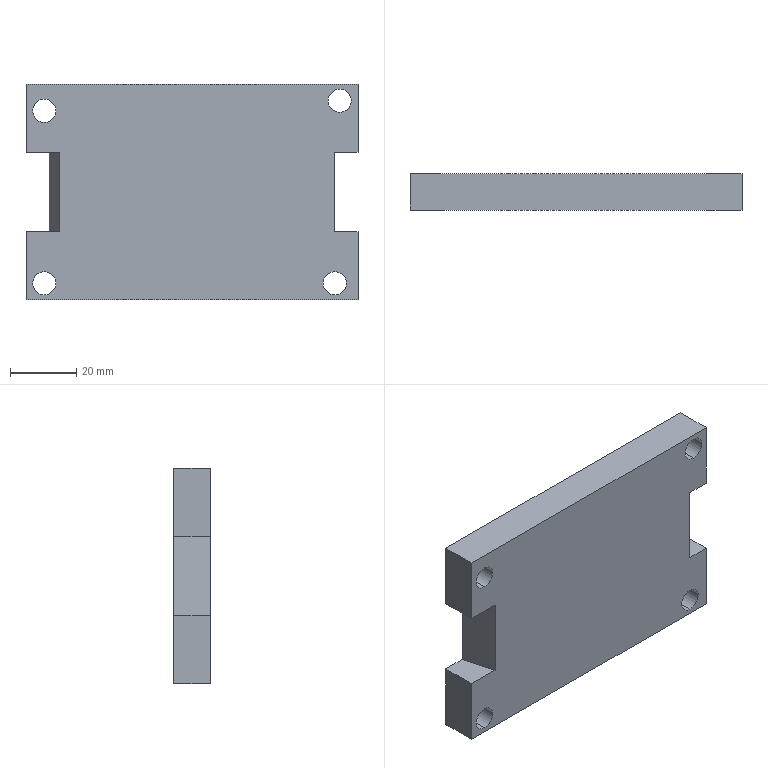Part | STEP file | X77ZZ-01001 | 1 solid | 22 faces | box 100 x 11 x 65 mm | volume 65319 mm3 | plane 14 | cylinder 8 | commonest cylinder face diameters 7 x8
STEP:
#1=CARTESIAN_POINT('',(-44.5,0.,-31.));
#2=VERTEX_POINT('',#1);
#3=CARTESIAN_POINT('',(-44.5,0.,-24.));
#4=VERTEX_POINT('',#3);
#5=CARTESIAN_POINT('',(-44.5,0.,-27.5));
#6=DIRECTION('',(0.,1.,0.));
#7=DIRECTION('',(0.,0.,1.));
#8=AXIS2_PLACEMENT_3D('',#5,#6,#7);
#9=CIRCLE('',#8,3.5);
#10=EDGE_CURVE('',#2,#4,#9,.T.);
#11=ORIENTED_EDGE('',*,*,#10,.F.);
#12=CARTESIAN_POINT('',(-44.5,11.,-31.));
#13=VERTEX_POINT('',#12);
#14=CARTESIAN_POINT('',(-44.5,0.,-31.));
#15=DIRECTION('',(0.,1.,0.));
#16=VECTOR('',#15,1000.);
#17=LINE('',#14,#16);
#18=EDGE_CURVE('',#2,#13,#17,.T.);
#19=ORIENTED_EDGE('',*,*,#18,.T.);
#20=CARTESIAN_POINT('',(-44.5,11.,-24.));
#21=VERTEX_POINT('',#20);
#22=CARTESIAN_POINT('',(-44.5,11.,-27.5));
#23=DIRECTION('',(0.,1.,0.));
#24=DIRECTION('',(0.,0.,1.));
#25=AXIS2_PLACEMENT_3D('',#22,#23,#24);
#26=CIRCLE('',#25,3.5);
#27=EDGE_CURVE('',#13,#21,#26,.T.);
#28=ORIENTED_EDGE('',*,*,#27,.T.);
#29=CARTESIAN_POINT('',(-44.5,0.,-24.));
#30=DIRECTION('',(0.,1.,0.));
#31=VECTOR('',#30,1000.);
#32=LINE('',#29,#31);
#33=EDGE_CURVE('',#4,#21,#32,.T.);
#34=ORIENTED_EDGE('',*,*,#33,.F.);
#35=EDGE_LOOP('',(#11,#19,#28,#34));
#36=FACE_OUTER_BOUND('',#35,.T.);
#37=CARTESIAN_POINT('',(-44.5,0.,-27.5));
#38=DIRECTION('',(0.,1.,0.));
#39=DIRECTION('',(0.,0.,1.));
#40=AXIS2_PLACEMENT_3D('',#37,#38,#39);
#41=CYLINDRICAL_SURFACE('',#40,3.5);
#42=ADVANCED_FACE('',(#36),#41,.F.);
#43=CARTESIAN_POINT('',(43.014,0.,-31.));
#44=VERTEX_POINT('',#43);
#45=CARTESIAN_POINT('',(43.014,0.,-24.));
#46=VERTEX_POINT('',#45);
#47=CARTESIAN_POINT('',(43.014,0.,-27.5));
#48=DIRECTION('',(0.,1.,0.));
#49=DIRECTION('',(0.,0.,1.));
#50=AXIS2_PLACEMENT_3D('',#47,#48,#49);
#51=CIRCLE('',#50,3.5);
#52=EDGE_CURVE('',#44,#46,#51,.T.);
#53=ORIENTED_EDGE('',*,*,#52,.F.);
#54=CARTESIAN_POINT('',(43.014,11.,-31.));
#55=VERTEX_POINT('',#54);
#56=CARTESIAN_POINT('',(43.014,0.,-31.));
#57=DIRECTION('',(0.,1.,0.));
#58=VECTOR('',#57,1000.);
#59=LINE('',#56,#58);
#60=EDGE_CURVE('',#44,#55,#59,.T.);
#61=ORIENTED_EDGE('',*,*,#60,.T.);
#62=CARTESIAN_POINT('',(43.014,11.,-24.));
#63=VERTEX_POINT('',#62);
#64=CARTESIAN_POINT('',(43.014,11.,-27.5));
#65=DIRECTION('',(0.,1.,0.));
#66=DIRECTION('',(0.,0.,1.));
#67=AXIS2_PLACEMENT_3D('',#64,#65,#66);
#68=CIRCLE('',#67,3.5);
#69=EDGE_CURVE('',#55,#63,#68,.T.);
#70=ORIENTED_EDGE('',*,*,#69,.T.);
#71=CARTESIAN_POINT('',(43.014,0.,-24.));
#72=DIRECTION('',(0.,1.,0.));
#73=VECTOR('',#72,1000.);
#74=LINE('',#71,#73);
#75=EDGE_CURVE('',#46,#63,#74,.T.);
#76=ORIENTED_EDGE('',*,*,#75,.F.);
#77=EDGE_LOOP('',(#53,#61,#70,#76));
#78=FACE_OUTER_BOUND('',#77,.T.);
#79=CARTESIAN_POINT('',(43.014,0.,-27.5));
#80=DIRECTION('',(0.,1.,0.));
#81=DIRECTION('',(0.,0.,1.));
#82=AXIS2_PLACEMENT_3D('',#79,#80,#81);
#83=CYLINDRICAL_SURFACE('',#82,3.5);
#84=ADVANCED_FACE('',(#78),#83,.F.);
#85=CARTESIAN_POINT('',(-44.5,0.,20.979));
#86=VERTEX_POINT('',#85);
#87=CARTESIAN_POINT('',(-44.5,0.,27.979));
#88=VERTEX_POINT('',#87);
#89=CARTESIAN_POINT('',(-44.5,0.,24.479));
#90=DIRECTION('',(0.,1.,0.));
#91=DIRECTION('',(0.,0.,1.));
#92=AXIS2_PLACEMENT_3D('',#89,#90,#91);
#93=CIRCLE('',#92,3.5);
#94=EDGE_CURVE('',#86,#88,#93,.T.);
#95=ORIENTED_EDGE('',*,*,#94,.F.);
#96=CARTESIAN_POINT('',(-44.5,11.,20.979));
#97=VERTEX_POINT('',#96);
#98=CARTESIAN_POINT('',(-44.5,0.,20.979));
#99=DIRECTION('',(0.,1.,0.));
#100=VECTOR('',#99,1000.);
#101=LINE('',#98,#100);
#102=EDGE_CURVE('',#86,#97,#101,.T.);
#103=ORIENTED_EDGE('',*,*,#102,.T.);
#104=CARTESIAN_POINT('',(-44.5,11.,27.979));
#105=VERTEX_POINT('',#104);
#106=CARTESIAN_POINT('',(-44.5,11.,24.479));
#107=DIRECTION('',(0.,1.,0.));
#108=DIRECTION('',(0.,0.,1.));
#109=AXIS2_PLACEMENT_3D('',#106,#107,#108);
#110=CIRCLE('',#109,3.5);
#111=EDGE_CURVE('',#97,#105,#110,.T.);
#112=ORIENTED_EDGE('',*,*,#111,.T.);
#113=CARTESIAN_POINT('',(-44.5,0.,27.979));
#114=DIRECTION('',(0.,1.,0.));
#115=VECTOR('',#114,1000.);
#116=LINE('',#113,#115);
#117=EDGE_CURVE('',#88,#105,#116,.T.);
#118=ORIENTED_EDGE('',*,*,#117,.F.);
#119=EDGE_LOOP('',(#95,#103,#112,#118));
#120=FACE_OUTER_BOUND('',#119,.T.);
#121=CARTESIAN_POINT('',(-44.5,0.,24.479));
#122=DIRECTION('',(0.,1.,0.));
#123=DIRECTION('',(0.,0.,1.));
#124=AXIS2_PLACEMENT_3D('',#121,#122,#123);
#125=CYLINDRICAL_SURFACE('',#124,3.5);
#126=ADVANCED_FACE('',(#120),#125,.F.);
#127=CARTESIAN_POINT('',(44.5,0.,24.));
#128=VERTEX_POINT('',#127);
#129=CARTESIAN_POINT('',(44.5,0.,31.));
#130=VERTEX_POINT('',#129);
#131=CARTESIAN_POINT('',(44.5,0.,27.5));
#132=DIRECTION('',(0.,1.,0.));
#133=DIRECTION('',(0.,0.,1.));
#134=AXIS2_PLACEMENT_3D('',#131,#132,#133);
#135=CIRCLE('',#134,3.5);
#136=EDGE_CURVE('',#128,#130,#135,.T.);
#137=ORIENTED_EDGE('',*,*,#136,.F.);
#138=CARTESIAN_POINT('',(44.5,11.,24.));
#139=VERTEX_POINT('',#138);
#140=CARTESIAN_POINT('',(44.5,0.,24.));
#141=DIRECTION('',(0.,1.,0.));
#142=VECTOR('',#141,1000.);
#143=LINE('',#140,#142);
#144=EDGE_CURVE('',#128,#139,#143,.T.);
#145=ORIENTED_EDGE('',*,*,#144,.T.);
#146=CARTESIAN_POINT('',(44.5,11.,31.));
#147=VERTEX_POINT('',#146);
#148=CARTESIAN_POINT('',(44.5,11.,27.5));
#149=DIRECTION('',(0.,1.,0.));
#150=DIRECTION('',(0.,0.,1.));
#151=AXIS2_PLACEMENT_3D('',#148,#149,#150);
#152=CIRCLE('',#151,3.5);
#153=EDGE_CURVE('',#139,#147,#152,.T.);
#154=ORIENTED_EDGE('',*,*,#153,.T.);
#155=CARTESIAN_POINT('',(44.5,0.,31.));
#156=DIRECTION('',(0.,1.,0.));
#157=VECTOR('',#156,1000.);
#158=LINE('',#155,#157);
#159=EDGE_CURVE('',#130,#147,#158,.T.);
#160=ORIENTED_EDGE('',*,*,#159,.F.);
#161=EDGE_LOOP('',(#137,#145,#154,#160));
#162=FACE_OUTER_BOUND('',#161,.T.);
#163=CARTESIAN_POINT('',(44.5,0.,27.5));
#164=DIRECTION('',(0.,1.,0.));
#165=DIRECTION('',(0.,0.,1.));
#166=AXIS2_PLACEMENT_3D('',#163,#164,#165);
#167=CYLINDRICAL_SURFACE('',#166,3.5);
#168=ADVANCED_FACE('',(#162),#167,.F.);
#169=CARTESIAN_POINT('',(-44.5,11.,-27.5));
#170=DIRECTION('',(0.,1.,0.));
#171=DIRECTION('',(0.,0.,1.));
#172=AXIS2_PLACEMENT_3D('',#169,#170,#171);
#173=CIRCLE('',#172,3.5);
#174=EDGE_CURVE('',#21,#13,#173,.T.);
#175=ORIENTED_EDGE('',*,*,#174,.F.);
#176=ORIENTED_EDGE('',*,*,#27,.F.);
#177=EDGE_LOOP('',(#175,#176));
#178=FACE_BOUND('',#177,.T.);
#179=CARTESIAN_POINT('',(43.014,11.,-27.5));
#180=DIRECTION('',(0.,1.,0.));
#181=DIRECTION('',(0.,0.,1.));
#182=AXIS2_PLACEMENT_3D('',#179,#180,#181);
#183=CIRCLE('',#182,3.5);
#184=EDGE_CURVE('',#63,#55,#183,.T.);
#185=ORIENTED_EDGE('',*,*,#184,.F.);
#186=ORIENTED_EDGE('',*,*,#69,.F.);
#187=EDGE_LOOP('',(#185,#186));
#188=FACE_BOUND('',#187,.T.);
#189=CARTESIAN_POINT('',(-44.5,11.,24.479));
#190=DIRECTION('',(0.,1.,0.));
#191=DIRECTION('',(0.,0.,1.));
#192=AXIS2_PLACEMENT_3D('',#189,#190,#191);
#193=CIRCLE('',#192,3.5);
#194=EDGE_CURVE('',#105,#97,#193,.T.);
#195=ORIENTED_EDGE('',*,*,#194,.F.);
#196=ORIENTED_EDGE('',*,*,#111,.F.);
#197=EDGE_LOOP('',(#195,#196));
#198=FACE_BOUND('',#197,.T.);
#199=CARTESIAN_POINT('',(44.5,11.,27.5));
#200=DIRECTION('',(0.,1.,0.));
#201=DIRECTION('',(0.,0.,1.));
#202=AXIS2_PLACEMENT_3D('',#199,#200,#201);
#203=CIRCLE('',#202,3.5);
#204=EDGE_CURVE('',#147,#139,#203,.T.);
#205=ORIENTED_EDGE('',*,*,#204,.F.);
#206=ORIENTED_EDGE('',*,*,#153,.F.);
#207=EDGE_LOOP('',(#205,#206));
#208=FACE_BOUND('',#207,.T.);
#209=CARTESIAN_POINT('',(-43.,11.,12.));
#210=VERTEX_POINT('',#209);
#211=CARTESIAN_POINT('',(-50.,11.,12.));
#212=VERTEX_POINT('',#211);
#213=CARTESIAN_POINT('',(-50.,11.,12.));
#214=DIRECTION('',(-1.,0.,0.));
#215=VECTOR('',#214,1000.);
#216=LINE('',#213,#215);
#217=EDGE_CURVE('',#210,#212,#216,.T.);
#218=ORIENTED_EDGE('',*,*,#217,.T.);
#219=CARTESIAN_POINT('',(-50.,11.,32.5));
#220=VERTEX_POINT('',#219);
#221=CARTESIAN_POINT('',(-50.,11.,32.5));
#222=DIRECTION('',(0.,0.,1.));
#223=VECTOR('',#222,1000.);
#224=LINE('',#221,#223);
#225=EDGE_CURVE('',#212,#220,#224,.T.);
#226=ORIENTED_EDGE('',*,*,#225,.T.);
#227=CARTESIAN_POINT('',(50.,11.,32.5));
#228=VERTEX_POINT('',#227);
#229=CARTESIAN_POINT('',(-50.,11.,32.5));
#230=DIRECTION('',(1.,0.,0.));
#231=VECTOR('',#230,1000.);
#232=LINE('',#229,#231);
#233=EDGE_CURVE('',#220,#228,#232,.T.);
#234=ORIENTED_EDGE('',*,*,#233,.T.);
#235=CARTESIAN_POINT('',(50.,11.,12.));
#236=VERTEX_POINT('',#235);
#237=CARTESIAN_POINT('',(50.,11.,32.5));
#238=DIRECTION('',(0.,0.,-1.));
#239=VECTOR('',#238,1000.);
#240=LINE('',#237,#239);
#241=EDGE_CURVE('',#228,#236,#240,.T.);
#242=ORIENTED_EDGE('',*,*,#241,.T.);
#243=CARTESIAN_POINT('',(40.,11.,12.));
#244=VERTEX_POINT('',#243);
#245=CARTESIAN_POINT('',(40.,11.,12.));
#246=DIRECTION('',(-1.,0.,0.));
#247=VECTOR('',#246,1000.);
#248=LINE('',#245,#247);
#249=EDGE_CURVE('',#236,#244,#248,.T.);
#250=ORIENTED_EDGE('',*,*,#249,.T.);
#251=CARTESIAN_POINT('',(40.,11.,-12.));
#252=VERTEX_POINT('',#251);
#253=CARTESIAN_POINT('',(40.,11.,12.));
#254=DIRECTION('',(0.,0.,-1.));
#255=VECTOR('',#254,1000.);
#256=LINE('',#253,#255);
#257=EDGE_CURVE('',#244,#252,#256,.T.);
#258=ORIENTED_EDGE('',*,*,#257,.T.);
#259=CARTESIAN_POINT('',(50.,11.,-12.));
#260=VERTEX_POINT('',#259);
#261=CARTESIAN_POINT('',(40.,11.,-12.));
#262=DIRECTION('',(-1.,0.,0.));
#263=VECTOR('',#262,1000.);
#264=LINE('',#261,#263);
#265=EDGE_CURVE('',#260,#252,#264,.T.);
#266=ORIENTED_EDGE('',*,*,#265,.F.);
#267=CARTESIAN_POINT('',(50.,11.,-32.5));
#268=VERTEX_POINT('',#267);
#269=CARTESIAN_POINT('',(50.,11.,32.5));
#270=DIRECTION('',(0.,0.,-1.));
#271=VECTOR('',#270,1000.);
#272=LINE('',#269,#271);
#273=EDGE_CURVE('',#260,#268,#272,.T.);
#274=ORIENTED_EDGE('',*,*,#273,.T.);
#275=CARTESIAN_POINT('',(-50.,11.,-32.5));
#276=VERTEX_POINT('',#275);
#277=CARTESIAN_POINT('',(-50.,11.,-32.5));
#278=DIRECTION('',(-1.,0.,0.));
#279=VECTOR('',#278,1000.);
#280=LINE('',#277,#279);
#281=EDGE_CURVE('',#268,#276,#280,.T.);
#282=ORIENTED_EDGE('',*,*,#281,.T.);
#283=CARTESIAN_POINT('',(-50.,11.,-12.));
#284=VERTEX_POINT('',#283);
#285=CARTESIAN_POINT('',(-50.,11.,32.5));
#286=DIRECTION('',(0.,0.,1.));
#287=VECTOR('',#286,1000.);
#288=LINE('',#285,#287);
#289=EDGE_CURVE('',#276,#284,#288,.T.);
#290=ORIENTED_EDGE('',*,*,#289,.T.);
#291=CARTESIAN_POINT('',(-43.,11.,-12.));
#292=VERTEX_POINT('',#291);
#293=CARTESIAN_POINT('',(-50.,11.,-12.));
#294=DIRECTION('',(-1.,0.,0.));
#295=VECTOR('',#294,1000.);
#296=LINE('',#293,#295);
#297=EDGE_CURVE('',#292,#284,#296,.T.);
#298=ORIENTED_EDGE('',*,*,#297,.F.);
#299=CARTESIAN_POINT('',(-43.,11.,12.));
#300=DIRECTION('',(0.,0.,-1.));
#301=VECTOR('',#300,1000.);
#302=LINE('',#299,#301);
#303=EDGE_CURVE('',#210,#292,#302,.T.);
#304=ORIENTED_EDGE('',*,*,#303,.F.);
#305=EDGE_LOOP('',(#218,#226,#234,#242,#250,#258,#266,#274,#282,#290,#298,#304));
#306=FACE_OUTER_BOUND('',#305,.T.);
#307=CARTESIAN_POINT('',(50.,11.,-32.5));
#308=DIRECTION('',(0.,-1.,0.));
#309=DIRECTION('',(0.,0.,-1.));
#310=AXIS2_PLACEMENT_3D('',#307,#308,#309);
#311=PLANE('',#310);
#312=ADVANCED_FACE('',(#178,#188,#198,#208,#306),#311,.F.);
#313=CARTESIAN_POINT('',(-44.5,0.,-27.5));
#314=DIRECTION('',(0.,1.,0.));
#315=DIRECTION('',(0.,0.,1.));
#316=AXIS2_PLACEMENT_3D('',#313,#314,#315);
#317=CIRCLE('',#316,3.5);
#318=EDGE_CURVE('',#4,#2,#317,.T.);
#319=ORIENTED_EDGE('',*,*,#318,.T.);
#320=ORIENTED_EDGE('',*,*,#10,.T.);
#321=EDGE_LOOP('',(#319,#320));
#322=FACE_BOUND('',#321,.T.);
#323=CARTESIAN_POINT('',(43.014,0.,-27.5));
#324=DIRECTION('',(0.,1.,0.));
#325=DIRECTION('',(0.,0.,1.));
#326=AXIS2_PLACEMENT_3D('',#323,#324,#325);
#327=CIRCLE('',#326,3.5);
#328=EDGE_CURVE('',#46,#44,#327,.T.);
#329=ORIENTED_EDGE('',*,*,#328,.T.);
#330=ORIENTED_EDGE('',*,*,#52,.T.);
#331=EDGE_LOOP('',(#329,#330));
#332=FACE_BOUND('',#331,.T.);
#333=CARTESIAN_POINT('',(-44.5,0.,24.479));
#334=DIRECTION('',(0.,1.,0.));
#335=DIRECTION('',(0.,0.,1.));
#336=AXIS2_PLACEMENT_3D('',#333,#334,#335);
#337=CIRCLE('',#336,3.5);
#338=EDGE_CURVE('',#88,#86,#337,.T.);
#339=ORIENTED_EDGE('',*,*,#338,.T.);
#340=ORIENTED_EDGE('',*,*,#94,.T.);
#341=EDGE_LOOP('',(#339,#340));
#342=FACE_BOUND('',#341,.T.);
#343=CARTESIAN_POINT('',(44.5,0.,27.5));
#344=DIRECTION('',(0.,1.,0.));
#345=DIRECTION('',(0.,0.,1.));
#346=AXIS2_PLACEMENT_3D('',#343,#344,#345);
#347=CIRCLE('',#346,3.5);
#348=EDGE_CURVE('',#130,#128,#347,.T.);
#349=ORIENTED_EDGE('',*,*,#348,.T.);
#350=ORIENTED_EDGE('',*,*,#136,.T.);
#351=EDGE_LOOP('',(#349,#350));
#352=FACE_BOUND('',#351,.T.);
#353=CARTESIAN_POINT('',(-50.,0.,12.));
#354=VERTEX_POINT('',#353);
#355=CARTESIAN_POINT('',(-50.,0.,32.5));
#356=VERTEX_POINT('',#355);
#357=CARTESIAN_POINT('',(-50.,0.,32.5));
#358=DIRECTION('',(0.,0.,1.));
#359=VECTOR('',#358,1000.);
#360=LINE('',#357,#359);
#361=EDGE_CURVE('',#354,#356,#360,.T.);
#362=ORIENTED_EDGE('',*,*,#361,.F.);
#363=CARTESIAN_POINT('',(-40.,0.,12.));
#364=VERTEX_POINT('',#363);
#365=CARTESIAN_POINT('',(-40.,0.,12.));
#366=DIRECTION('',(1.,0.,0.));
#367=VECTOR('',#366,1000.);
#368=LINE('',#365,#367);
#369=EDGE_CURVE('',#354,#364,#368,.T.);
#370=ORIENTED_EDGE('',*,*,#369,.T.);
#371=CARTESIAN_POINT('',(-40.,0.,-12.));
#372=VERTEX_POINT('',#371);
#373=CARTESIAN_POINT('',(-40.,0.,12.));
#374=DIRECTION('',(0.,0.,-1.));
#375=VECTOR('',#374,1000.);
#376=LINE('',#373,#375);
#377=EDGE_CURVE('',#364,#372,#376,.T.);
#378=ORIENTED_EDGE('',*,*,#377,.T.);
#379=CARTESIAN_POINT('',(-50.,0.,-12.));
#380=VERTEX_POINT('',#379);
#381=CARTESIAN_POINT('',(-40.,0.,-12.));
#382=DIRECTION('',(1.,0.,0.));
#383=VECTOR('',#382,1000.);
#384=LINE('',#381,#383);
#385=EDGE_CURVE('',#380,#372,#384,.T.);
#386=ORIENTED_EDGE('',*,*,#385,.F.);
#387=CARTESIAN_POINT('',(-50.,0.,-32.5));
#388=VERTEX_POINT('',#387);
#389=CARTESIAN_POINT('',(-50.,0.,32.5));
#390=DIRECTION('',(0.,0.,1.));
#391=VECTOR('',#390,1000.);
#392=LINE('',#389,#391);
#393=EDGE_CURVE('',#388,#380,#392,.T.);
#394=ORIENTED_EDGE('',*,*,#393,.F.);
#395=CARTESIAN_POINT('',(50.,0.,-32.5));
#396=VERTEX_POINT('',#395);
#397=CARTESIAN_POINT('',(-50.,0.,-32.5));
#398=DIRECTION('',(-1.,0.,0.));
#399=VECTOR('',#398,1000.);
#400=LINE('',#397,#399);
#401=EDGE_CURVE('',#396,#388,#400,.T.);
#402=ORIENTED_EDGE('',*,*,#401,.F.);
#403=CARTESIAN_POINT('',(50.,0.,-12.));
#404=VERTEX_POINT('',#403);
#405=CARTESIAN_POINT('',(50.,0.,32.5));
#406=DIRECTION('',(0.,0.,-1.));
#407=VECTOR('',#406,1000.);
#408=LINE('',#405,#407);
#409=EDGE_CURVE('',#404,#396,#408,.T.);
#410=ORIENTED_EDGE('',*,*,#409,.F.);
#411=CARTESIAN_POINT('',(43.,0.,-12.));
#412=VERTEX_POINT('',#411);
#413=CARTESIAN_POINT('',(50.,0.,-12.));
#414=DIRECTION('',(1.,0.,0.));
#415=VECTOR('',#414,1000.);
#416=LINE('',#413,#415);
#417=EDGE_CURVE('',#412,#404,#416,.T.);
#418=ORIENTED_EDGE('',*,*,#417,.F.);
#419=CARTESIAN_POINT('',(43.,0.,12.));
#420=VERTEX_POINT('',#419);
#421=CARTESIAN_POINT('',(43.,0.,12.));
#422=DIRECTION('',(0.,0.,-1.));
#423=VECTOR('',#422,1000.);
#424=LINE('',#421,#423);
#425=EDGE_CURVE('',#420,#412,#424,.T.);
#426=ORIENTED_EDGE('',*,*,#425,.F.);
#427=CARTESIAN_POINT('',(50.,0.,12.));
#428=VERTEX_POINT('',#427);
#429=CARTESIAN_POINT('',(50.,0.,12.));
#430=DIRECTION('',(1.,0.,0.));
#431=VECTOR('',#430,1000.);
#432=LINE('',#429,#431);
#433=EDGE_CURVE('',#420,#428,#432,.T.);
#434=ORIENTED_EDGE('',*,*,#433,.T.);
#435=CARTESIAN_POINT('',(50.,0.,32.5));
#436=VERTEX_POINT('',#435);
#437=CARTESIAN_POINT('',(50.,0.,32.5));
#438=DIRECTION('',(0.,0.,-1.));
#439=VECTOR('',#438,1000.);
#440=LINE('',#437,#439);
#441=EDGE_CURVE('',#436,#428,#440,.T.);
#442=ORIENTED_EDGE('',*,*,#441,.F.);
#443=CARTESIAN_POINT('',(-50.,0.,32.5));
#444=DIRECTION('',(1.,0.,0.));
#445=VECTOR('',#444,1000.);
#446=LINE('',#443,#445);
#447=EDGE_CURVE('',#356,#436,#446,.T.);
#448=ORIENTED_EDGE('',*,*,#447,.F.);
#449=EDGE_LOOP('',(#362,#370,#378,#386,#394,#402,#410,#418,#426,#434,#442,#448));
#450=FACE_OUTER_BOUND('',#449,.T.);
#451=CARTESIAN_POINT('',(50.,0.,-32.5));
#452=DIRECTION('',(0.,-1.,0.));
#453=DIRECTION('',(0.,0.,-1.));
#454=AXIS2_PLACEMENT_3D('',#451,#452,#453);
#455=PLANE('',#454);
#456=ADVANCED_FACE('',(#322,#332,#342,#352,#450),#455,.T.);
#457=CARTESIAN_POINT('',(-50.,0.,12.));
#458=DIRECTION('',(0.,-1.,0.));
#459=VECTOR('',#458,1000.);
#460=LINE('',#457,#459);
#461=EDGE_CURVE('',#212,#354,#460,.T.);
#462=ORIENTED_EDGE('',*,*,#461,.T.);
#463=ORIENTED_EDGE('',*,*,#361,.T.);
#464=CARTESIAN_POINT('',(-50.,11.,32.5));
#465=DIRECTION('',(0.,-1.,0.));
#466=VECTOR('',#465,1000.);
#467=LINE('',#464,#466);
#468=EDGE_CURVE('',#220,#356,#467,.T.);
#469=ORIENTED_EDGE('',*,*,#468,.F.);
#470=ORIENTED_EDGE('',*,*,#225,.F.);
#471=EDGE_LOOP('',(#462,#463,#469,#470));
#472=FACE_OUTER_BOUND('',#471,.T.);
#473=CARTESIAN_POINT('',(-50.,11.,32.5));
#474=DIRECTION('',(1.,0.,0.));
#475=DIRECTION('',(0.,0.,-1.));
#476=AXIS2_PLACEMENT_3D('',#473,#474,#475);
#477=PLANE('',#476);
#478=ADVANCED_FACE('',(#472),#477,.F.);
#479=CARTESIAN_POINT('',(50.,11.,12.));
#480=DIRECTION('',(0.,1.,0.));
#481=VECTOR('',#480,1000.);
#482=LINE('',#479,#481);
#483=EDGE_CURVE('',#428,#236,#482,.T.);
#484=ORIENTED_EDGE('',*,*,#483,.T.);
#485=ORIENTED_EDGE('',*,*,#241,.F.);
#486=CARTESIAN_POINT('',(50.,11.,32.5));
#487=DIRECTION('',(0.,-1.,0.));
#488=VECTOR('',#487,1000.);
#489=LINE('',#486,#488);
#490=EDGE_CURVE('',#228,#436,#489,.T.);
#491=ORIENTED_EDGE('',*,*,#490,.T.);
#492=ORIENTED_EDGE('',*,*,#441,.T.);
#493=EDGE_LOOP('',(#484,#485,#491,#492));
#494=FACE_OUTER_BOUND('',#493,.T.);
#495=CARTESIAN_POINT('',(50.,11.,32.5));
#496=DIRECTION('',(-1.,0.,0.));
#497=DIRECTION('',(0.,0.,1.));
#498=AXIS2_PLACEMENT_3D('',#495,#496,#497);
#499=PLANE('',#498);
#500=ADVANCED_FACE('',(#494),#499,.F.);
#501=ORIENTED_EDGE('',*,*,#273,.F.);
#502=CARTESIAN_POINT('',(50.,11.,-12.));
#503=DIRECTION('',(0.,1.,0.));
#504=VECTOR('',#503,1000.);
#505=LINE('',#502,#504);
#506=EDGE_CURVE('',#404,#260,#505,.T.);
#507=ORIENTED_EDGE('',*,*,#506,.F.);
#508=ORIENTED_EDGE('',*,*,#409,.T.);
#509=CARTESIAN_POINT('',(50.,11.,-32.5));
#510=DIRECTION('',(0.,-1.,0.));
#511=VECTOR('',#510,1000.);
#512=LINE('',#509,#511);
#513=EDGE_CURVE('',#268,#396,#512,.T.);
#514=ORIENTED_EDGE('',*,*,#513,.F.);
#515=EDGE_LOOP('',(#501,#507,#508,#514));
#516=FACE_OUTER_BOUND('',#515,.T.);
#517=CARTESIAN_POINT('',(50.,11.,32.5));
#518=DIRECTION('',(-1.,0.,0.));
#519=DIRECTION('',(0.,0.,1.));
#520=AXIS2_PLACEMENT_3D('',#517,#518,#519);
#521=PLANE('',#520);
#522=ADVANCED_FACE('',(#516),#521,.F.);
#523=ORIENTED_EDGE('',*,*,#401,.T.);
#524=CARTESIAN_POINT('',(-50.,11.,-32.5));
#525=DIRECTION('',(0.,-1.,0.));
#526=VECTOR('',#525,1000.);
#527=LINE('',#524,#526);
#528=EDGE_CURVE('',#276,#388,#527,.T.);
#529=ORIENTED_EDGE('',*,*,#528,.F.);
#530=ORIENTED_EDGE('',*,*,#281,.F.);
#531=ORIENTED_EDGE('',*,*,#513,.T.);
#532=EDGE_LOOP('',(#523,#529,#530,#531));
#533=FACE_OUTER_BOUND('',#532,.T.);
#534=CARTESIAN_POINT('',(-50.,11.,-32.5));
#535=DIRECTION('',(0.,0.,1.));
#536=DIRECTION('',(1.,0.,0.));
#537=AXIS2_PLACEMENT_3D('',#534,#535,#536);
#538=PLANE('',#537);
#539=ADVANCED_FACE('',(#533),#538,.F.);
#540=ORIENTED_EDGE('',*,*,#393,.T.);
#541=CARTESIAN_POINT('',(-50.,0.,-12.));
#542=DIRECTION('',(0.,-1.,0.));
#543=VECTOR('',#542,1000.);
#544=LINE('',#541,#543);
#545=EDGE_CURVE('',#284,#380,#544,.T.);
#546=ORIENTED_EDGE('',*,*,#545,.F.);
#547=ORIENTED_EDGE('',*,*,#289,.F.);
#548=ORIENTED_EDGE('',*,*,#528,.T.);
#549=EDGE_LOOP('',(#540,#546,#547,#548));
#550=FACE_OUTER_BOUND('',#549,.T.);
#551=CARTESIAN_POINT('',(-50.,11.,32.5));
#552=DIRECTION('',(1.,0.,0.));
#553=DIRECTION('',(0.,0.,-1.));
#554=AXIS2_PLACEMENT_3D('',#551,#552,#553);
#555=PLANE('',#554);
#556=ADVANCED_FACE('',(#550),#555,.F.);
#557=ORIENTED_EDGE('',*,*,#447,.T.);
#558=ORIENTED_EDGE('',*,*,#490,.F.);
#559=ORIENTED_EDGE('',*,*,#233,.F.);
#560=ORIENTED_EDGE('',*,*,#468,.T.);
#561=EDGE_LOOP('',(#557,#558,#559,#560));
#562=FACE_OUTER_BOUND('',#561,.T.);
#563=CARTESIAN_POINT('',(-50.,11.,32.5));
#564=DIRECTION('',(0.,0.,-1.));
#565=DIRECTION('',(-1.,0.,0.));
#566=AXIS2_PLACEMENT_3D('',#563,#564,#565);
#567=PLANE('',#566);
#568=ADVANCED_FACE('',(#562),#567,.F.);
#569=ORIENTED_EDGE('',*,*,#257,.F.);
#570=CARTESIAN_POINT('',(40.,11.,12.));
#571=DIRECTION('',(0.2631,-0.9648,0.));
#572=VECTOR('',#571,1000.);
#573=LINE('',#570,#572);
#574=EDGE_CURVE('',#244,#420,#573,.T.);
#575=ORIENTED_EDGE('',*,*,#574,.T.);
#576=ORIENTED_EDGE('',*,*,#425,.T.);
#577=CARTESIAN_POINT('',(40.,11.,-12.));
#578=DIRECTION('',(0.2631,-0.9648,0.));
#579=VECTOR('',#578,1000.);
#580=LINE('',#577,#579);
#581=EDGE_CURVE('',#252,#412,#580,.T.);
#582=ORIENTED_EDGE('',*,*,#581,.F.);
#583=EDGE_LOOP('',(#569,#575,#576,#582));
#584=FACE_OUTER_BOUND('',#583,.T.);
#585=CARTESIAN_POINT('',(40.,11.,12.));
#586=DIRECTION('',(0.9648,0.2631,0.));
#587=DIRECTION('',(-0.2631,0.9648,0.));
#588=AXIS2_PLACEMENT_3D('',#585,#586,#587);
#589=PLANE('',#588);
#590=ADVANCED_FACE('',(#584),#589,.T.);
#591=ORIENTED_EDGE('',*,*,#249,.F.);
#592=ORIENTED_EDGE('',*,*,#483,.F.);
#593=ORIENTED_EDGE('',*,*,#433,.F.);
#594=ORIENTED_EDGE('',*,*,#574,.F.);
#595=EDGE_LOOP('',(#591,#592,#593,#594));
#596=FACE_OUTER_BOUND('',#595,.T.);
#597=CARTESIAN_POINT('',(50.,11.,12.));
#598=DIRECTION('',(0.,0.,-1.));
#599=DIRECTION('',(-1.,0.,0.));
#600=AXIS2_PLACEMENT_3D('',#597,#598,#599);
#601=PLANE('',#600);
#602=ADVANCED_FACE('',(#596),#601,.T.);
#603=ORIENTED_EDGE('',*,*,#265,.T.);
#604=ORIENTED_EDGE('',*,*,#581,.T.);
#605=ORIENTED_EDGE('',*,*,#417,.T.);
#606=ORIENTED_EDGE('',*,*,#506,.T.);
#607=EDGE_LOOP('',(#603,#604,#605,#606));
#608=FACE_OUTER_BOUND('',#607,.T.);
#609=CARTESIAN_POINT('',(50.,11.,-12.));
#610=DIRECTION('',(0.,0.,-1.));
#611=DIRECTION('',(-1.,0.,0.));
#612=AXIS2_PLACEMENT_3D('',#609,#610,#611);
#613=PLANE('',#612);
#614=ADVANCED_FACE('',(#608),#613,.F.);
#615=ORIENTED_EDGE('',*,*,#377,.F.);
#616=CARTESIAN_POINT('',(-43.,11.,12.));
#617=DIRECTION('',(-0.2631,0.9648,0.));
#618=VECTOR('',#617,1000.);
#619=LINE('',#616,#618);
#620=EDGE_CURVE('',#364,#210,#619,.T.);
#621=ORIENTED_EDGE('',*,*,#620,.T.);
#622=ORIENTED_EDGE('',*,*,#303,.T.);
#623=CARTESIAN_POINT('',(-43.,11.,-12.));
#624=DIRECTION('',(-0.2631,0.9648,0.));
#625=VECTOR('',#624,1000.);
#626=LINE('',#623,#625);
#627=EDGE_CURVE('',#372,#292,#626,.T.);
#628=ORIENTED_EDGE('',*,*,#627,.F.);
#629=EDGE_LOOP('',(#615,#621,#622,#628));
#630=FACE_OUTER_BOUND('',#629,.T.);
#631=CARTESIAN_POINT('',(-43.,11.,12.));
#632=DIRECTION('',(-0.9648,-0.2631,0.));
#633=DIRECTION('',(0.2631,-0.9648,0.));
#634=AXIS2_PLACEMENT_3D('',#631,#632,#633);
#635=PLANE('',#634);
#636=ADVANCED_FACE('',(#630),#635,.T.);
#637=ORIENTED_EDGE('',*,*,#461,.F.);
#638=ORIENTED_EDGE('',*,*,#217,.F.);
#639=ORIENTED_EDGE('',*,*,#620,.F.);
#640=ORIENTED_EDGE('',*,*,#369,.F.);
#641=EDGE_LOOP('',(#637,#638,#639,#640));
#642=FACE_OUTER_BOUND('',#641,.T.);
#643=CARTESIAN_POINT('',(-50.,11.,12.));
#644=DIRECTION('',(0.,0.,-1.));
#645=DIRECTION('',(-1.,0.,0.));
#646=AXIS2_PLACEMENT_3D('',#643,#644,#645);
#647=PLANE('',#646);
#648=ADVANCED_FACE('',(#642),#647,.T.);
#649=ORIENTED_EDGE('',*,*,#545,.T.);
#650=ORIENTED_EDGE('',*,*,#385,.T.);
#651=ORIENTED_EDGE('',*,*,#627,.T.);
#652=ORIENTED_EDGE('',*,*,#297,.T.);
#653=EDGE_LOOP('',(#649,#650,#651,#652));
#654=FACE_OUTER_BOUND('',#653,.T.);
#655=CARTESIAN_POINT('',(-50.,11.,-12.));
#656=DIRECTION('',(0.,0.,-1.));
#657=DIRECTION('',(-1.,0.,0.));
#658=AXIS2_PLACEMENT_3D('',#655,#656,#657);
#659=PLANE('',#658);
#660=ADVANCED_FACE('',(#654),#659,.F.);
#661=ORIENTED_EDGE('',*,*,#144,.F.);
#662=ORIENTED_EDGE('',*,*,#348,.F.);
#663=ORIENTED_EDGE('',*,*,#159,.T.);
#664=ORIENTED_EDGE('',*,*,#204,.T.);
#665=EDGE_LOOP('',(#661,#662,#663,#664));
#666=FACE_OUTER_BOUND('',#665,.T.);
#667=CARTESIAN_POINT('',(44.5,0.,27.5));
#668=DIRECTION('',(0.,1.,0.));
#669=DIRECTION('',(0.,0.,1.));
#670=AXIS2_PLACEMENT_3D('',#667,#668,#669);
#671=CYLINDRICAL_SURFACE('',#670,3.5);
#672=ADVANCED_FACE('',(#666),#671,.F.);
#673=ORIENTED_EDGE('',*,*,#102,.F.);
#674=ORIENTED_EDGE('',*,*,#338,.F.);
#675=ORIENTED_EDGE('',*,*,#117,.T.);
#676=ORIENTED_EDGE('',*,*,#194,.T.);
#677=EDGE_LOOP('',(#673,#674,#675,#676));
#678=FACE_OUTER_BOUND('',#677,.T.);
#679=CARTESIAN_POINT('',(-44.5,0.,24.479));
#680=DIRECTION('',(0.,1.,0.));
#681=DIRECTION('',(0.,0.,1.));
#682=AXIS2_PLACEMENT_3D('',#679,#680,#681);
#683=CYLINDRICAL_SURFACE('',#682,3.5);
#684=ADVANCED_FACE('',(#678),#683,.F.);
#685=ORIENTED_EDGE('',*,*,#60,.F.);
#686=ORIENTED_EDGE('',*,*,#328,.F.);
#687=ORIENTED_EDGE('',*,*,#75,.T.);
#688=ORIENTED_EDGE('',*,*,#184,.T.);
#689=EDGE_LOOP('',(#685,#686,#687,#688));
#690=FACE_OUTER_BOUND('',#689,.T.);
#691=CARTESIAN_POINT('',(43.014,0.,-27.5));
#692=DIRECTION('',(0.,1.,0.));
#693=DIRECTION('',(0.,0.,1.));
#694=AXIS2_PLACEMENT_3D('',#691,#692,#693);
#695=CYLINDRICAL_SURFACE('',#694,3.5);
#696=ADVANCED_FACE('',(#690),#695,.F.);
#697=ORIENTED_EDGE('',*,*,#18,.F.);
#698=ORIENTED_EDGE('',*,*,#318,.F.);
#699=ORIENTED_EDGE('',*,*,#33,.T.);
#700=ORIENTED_EDGE('',*,*,#174,.T.);
#701=EDGE_LOOP('',(#697,#698,#699,#700));
#702=FACE_OUTER_BOUND('',#701,.T.);
#703=CARTESIAN_POINT('',(-44.5,0.,-27.5));
#704=DIRECTION('',(0.,1.,0.));
#705=DIRECTION('',(0.,0.,1.));
#706=AXIS2_PLACEMENT_3D('',#703,#704,#705);
#707=CYLINDRICAL_SURFACE('',#706,3.5);
#708=ADVANCED_FACE('',(#702),#707,.F.);
#709=CLOSED_SHELL('',(#42,#84,#126,#168,#312,#456,#478,#500,#522,#539,#556,#568,#590,#602,#614,#636,#648,#660,#672,#684,#696,#708));
#710=MANIFOLD_SOLID_BREP('',#709);
#711=CARTESIAN_POINT('',(0.,0.,0.));
#712=DIRECTION('',(0.,0.,1.));
#713=DIRECTION('',(1.,0.,0.));
#714=AXIS2_PLACEMENT_3D('',#711,#712,#713);
#715=(LENGTH_UNIT()NAMED_UNIT(*)SI_UNIT(.MILLI.,.METRE.));
#716=UNCERTAINTY_MEASURE_WITH_UNIT(LENGTH_MEASURE(0.00001),#715,'','');
#717=(NAMED_UNIT(*)PLANE_ANGLE_UNIT()SI_UNIT($,.RADIAN.));
#718=(NAMED_UNIT(*)SI_UNIT($,.STERADIAN.)SOLID_ANGLE_UNIT());
#719=(GEOMETRIC_REPRESENTATION_CONTEXT(3)GLOBAL_UNCERTAINTY_ASSIGNED_CONTEXT((#716))GLOBAL_UNIT_ASSIGNED_CONTEXT((#715,#717,#718))REPRESENTATION_CONTEXT('',''));
#720=ADVANCED_BREP_SHAPE_REPRESENTATION('',(#710,#714),#719);